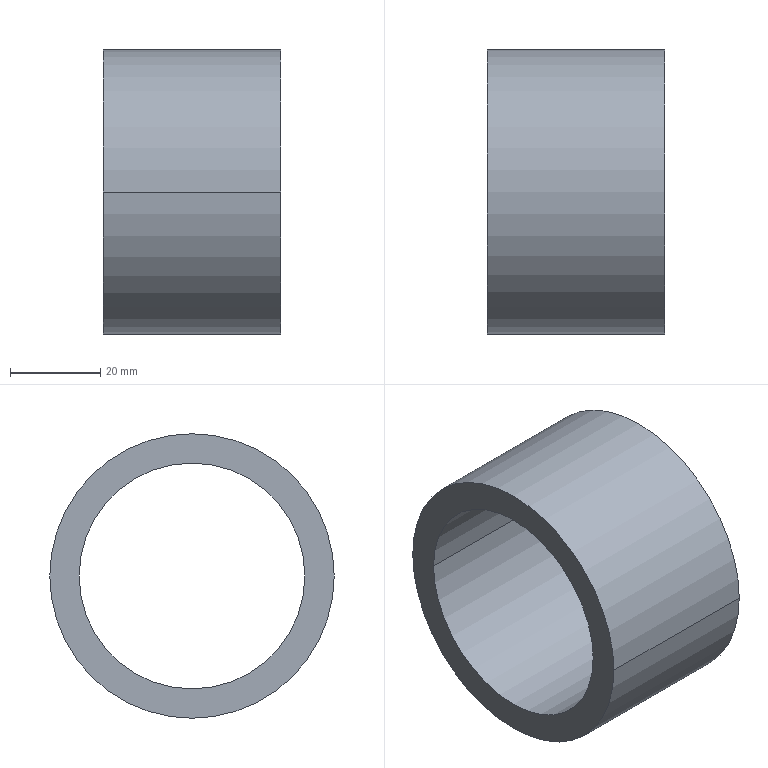Part | SolidWorks | features Extrusion 1 | 1 solid | 6 faces | box 39.25 x 63 x 63 mm | volume 45285 mm3 | cylinder 4 | plane 2 | commonest cylinder face diameters 50 x2 63 x2
STEP:
#1=CARTESIAN_POINT('',(231.,65.,-102.5));
#2=VERTEX_POINT('',#1);
#3=CARTESIAN_POINT('',(231.,115.,-102.5));
#4=VERTEX_POINT('',#3);
#5=CARTESIAN_POINT('',(231.,90.,-102.5));
#6=DIRECTION('',(1.,0.,0.));
#7=DIRECTION('',(0.,1.,0.));
#8=AXIS2_PLACEMENT_3D('',#5,#6,#7);
#9=CIRCLE('',#8,25.);
#10=EDGE_CURVE('',#2,#4,#9,.T.);
#11=ORIENTED_EDGE('',*,*,#10,.T.);
#12=CARTESIAN_POINT('',(191.75,115.,-102.5));
#13=VERTEX_POINT('',#12);
#14=CARTESIAN_POINT('',(231.,115.,-102.5));
#15=DIRECTION('',(-1.,0.,0.));
#16=VECTOR('',#15,1000.);
#17=LINE('',#14,#16);
#18=EDGE_CURVE('',#4,#13,#17,.T.);
#19=ORIENTED_EDGE('',*,*,#18,.T.);
#20=CARTESIAN_POINT('',(191.75,65.,-102.5));
#21=VERTEX_POINT('',#20);
#22=CARTESIAN_POINT('',(191.75,90.,-102.5));
#23=DIRECTION('',(1.,0.,0.));
#24=DIRECTION('',(0.,1.,0.));
#25=AXIS2_PLACEMENT_3D('',#22,#23,#24);
#26=CIRCLE('',#25,25.);
#27=EDGE_CURVE('',#21,#13,#26,.T.);
#28=ORIENTED_EDGE('',*,*,#27,.F.);
#29=CARTESIAN_POINT('',(231.,65.,-102.5));
#30=DIRECTION('',(-1.,0.,0.));
#31=VECTOR('',#30,1000.);
#32=LINE('',#29,#31);
#33=EDGE_CURVE('',#2,#21,#32,.T.);
#34=ORIENTED_EDGE('',*,*,#33,.F.);
#35=EDGE_LOOP('',(#11,#19,#28,#34));
#36=FACE_OUTER_BOUND('',#35,.T.);
#37=CARTESIAN_POINT('',(231.,90.,-102.5));
#38=DIRECTION('',(-1.,0.,0.));
#39=DIRECTION('',(0.,-1.,0.));
#40=AXIS2_PLACEMENT_3D('',#37,#38,#39);
#41=CYLINDRICAL_SURFACE('',#40,25.);
#42=ADVANCED_FACE('',(#36),#41,.F.);
#43=CARTESIAN_POINT('',(231.,121.5,-102.5));
#44=VERTEX_POINT('',#43);
#45=CARTESIAN_POINT('',(231.,58.5,-102.5));
#46=VERTEX_POINT('',#45);
#47=CARTESIAN_POINT('',(231.,90.,-102.5));
#48=DIRECTION('',(1.,0.,0.));
#49=DIRECTION('',(0.,1.,0.));
#50=AXIS2_PLACEMENT_3D('',#47,#48,#49);
#51=CIRCLE('',#50,31.5);
#52=EDGE_CURVE('',#44,#46,#51,.T.);
#53=ORIENTED_EDGE('',*,*,#52,.F.);
#54=CARTESIAN_POINT('',(191.75,121.5,-102.5));
#55=VERTEX_POINT('',#54);
#56=CARTESIAN_POINT('',(231.,121.5,-102.5));
#57=DIRECTION('',(-1.,0.,0.));
#58=VECTOR('',#57,1000.);
#59=LINE('',#56,#58);
#60=EDGE_CURVE('',#44,#55,#59,.T.);
#61=ORIENTED_EDGE('',*,*,#60,.T.);
#62=CARTESIAN_POINT('',(191.75,58.5,-102.5));
#63=VERTEX_POINT('',#62);
#64=CARTESIAN_POINT('',(191.75,90.,-102.5));
#65=DIRECTION('',(1.,0.,0.));
#66=DIRECTION('',(0.,1.,0.));
#67=AXIS2_PLACEMENT_3D('',#64,#65,#66);
#68=CIRCLE('',#67,31.5);
#69=EDGE_CURVE('',#55,#63,#68,.T.);
#70=ORIENTED_EDGE('',*,*,#69,.T.);
#71=CARTESIAN_POINT('',(231.,58.5,-102.5));
#72=DIRECTION('',(-1.,0.,0.));
#73=VECTOR('',#72,1000.);
#74=LINE('',#71,#73);
#75=EDGE_CURVE('',#46,#63,#74,.T.);
#76=ORIENTED_EDGE('',*,*,#75,.F.);
#77=EDGE_LOOP('',(#53,#61,#70,#76));
#78=FACE_OUTER_BOUND('',#77,.T.);
#79=CARTESIAN_POINT('',(231.,90.,-102.5));
#80=DIRECTION('',(-1.,0.,0.));
#81=DIRECTION('',(0.,-1.,0.));
#82=AXIS2_PLACEMENT_3D('',#79,#80,#81);
#83=CYLINDRICAL_SURFACE('',#82,31.5);
#84=ADVANCED_FACE('',(#78),#83,.T.);
#85=CARTESIAN_POINT('',(231.,90.,-102.5));
#86=DIRECTION('',(1.,0.,0.));
#87=DIRECTION('',(0.,1.,0.));
#88=AXIS2_PLACEMENT_3D('',#85,#86,#87);
#89=CIRCLE('',#88,31.5);
#90=EDGE_CURVE('',#46,#44,#89,.T.);
#91=ORIENTED_EDGE('',*,*,#90,.T.);
#92=ORIENTED_EDGE('',*,*,#52,.T.);
#93=EDGE_LOOP('',(#91,#92));
#94=FACE_OUTER_BOUND('',#93,.T.);
#95=ORIENTED_EDGE('',*,*,#10,.F.);
#96=CARTESIAN_POINT('',(231.,90.,-102.5));
#97=DIRECTION('',(1.,0.,0.));
#98=DIRECTION('',(0.,1.,0.));
#99=AXIS2_PLACEMENT_3D('',#96,#97,#98);
#100=CIRCLE('',#99,25.);
#101=EDGE_CURVE('',#4,#2,#100,.T.);
#102=ORIENTED_EDGE('',*,*,#101,.F.);
#103=EDGE_LOOP('',(#95,#102));
#104=FACE_BOUND('',#103,.T.);
#105=CARTESIAN_POINT('',(231.,90.,-102.5));
#106=DIRECTION('',(1.,0.,0.));
#107=DIRECTION('',(0.,1.,0.));
#108=AXIS2_PLACEMENT_3D('',#105,#106,#107);
#109=PLANE('',#108);
#110=ADVANCED_FACE('',(#94,#104),#109,.T.);
#111=CARTESIAN_POINT('',(191.75,90.,-102.5));
#112=DIRECTION('',(1.,0.,0.));
#113=DIRECTION('',(0.,1.,0.));
#114=AXIS2_PLACEMENT_3D('',#111,#112,#113);
#115=CIRCLE('',#114,31.5);
#116=EDGE_CURVE('',#63,#55,#115,.T.);
#117=ORIENTED_EDGE('',*,*,#116,.F.);
#118=ORIENTED_EDGE('',*,*,#69,.F.);
#119=EDGE_LOOP('',(#117,#118));
#120=FACE_OUTER_BOUND('',#119,.T.);
#121=ORIENTED_EDGE('',*,*,#27,.T.);
#122=CARTESIAN_POINT('',(191.75,90.,-102.5));
#123=DIRECTION('',(1.,0.,0.));
#124=DIRECTION('',(0.,1.,0.));
#125=AXIS2_PLACEMENT_3D('',#122,#123,#124);
#126=CIRCLE('',#125,25.);
#127=EDGE_CURVE('',#13,#21,#126,.T.);
#128=ORIENTED_EDGE('',*,*,#127,.T.);
#129=EDGE_LOOP('',(#121,#128));
#130=FACE_BOUND('',#129,.T.);
#131=CARTESIAN_POINT('',(191.75,90.,-102.5));
#132=DIRECTION('',(1.,0.,0.));
#133=DIRECTION('',(0.,1.,0.));
#134=AXIS2_PLACEMENT_3D('',#131,#132,#133);
#135=PLANE('',#134);
#136=ADVANCED_FACE('',(#120,#130),#135,.F.);
#137=ORIENTED_EDGE('',*,*,#60,.F.);
#138=ORIENTED_EDGE('',*,*,#90,.F.);
#139=ORIENTED_EDGE('',*,*,#75,.T.);
#140=ORIENTED_EDGE('',*,*,#116,.T.);
#141=EDGE_LOOP('',(#137,#138,#139,#140));
#142=FACE_OUTER_BOUND('',#141,.T.);
#143=CARTESIAN_POINT('',(231.,90.,-102.5));
#144=DIRECTION('',(-1.,0.,0.));
#145=DIRECTION('',(0.,-1.,0.));
#146=AXIS2_PLACEMENT_3D('',#143,#144,#145);
#147=CYLINDRICAL_SURFACE('',#146,31.5);
#148=ADVANCED_FACE('',(#142),#147,.T.);
#149=ORIENTED_EDGE('',*,*,#18,.F.);
#150=ORIENTED_EDGE('',*,*,#101,.T.);
#151=ORIENTED_EDGE('',*,*,#33,.T.);
#152=ORIENTED_EDGE('',*,*,#127,.F.);
#153=EDGE_LOOP('',(#149,#150,#151,#152));
#154=FACE_OUTER_BOUND('',#153,.T.);
#155=CARTESIAN_POINT('',(231.,90.,-102.5));
#156=DIRECTION('',(-1.,0.,0.));
#157=DIRECTION('',(0.,-1.,0.));
#158=AXIS2_PLACEMENT_3D('',#155,#156,#157);
#159=CYLINDRICAL_SURFACE('',#158,25.);
#160=ADVANCED_FACE('',(#154),#159,.F.);
#161=CLOSED_SHELL('',(#42,#84,#110,#136,#148,#160));
#162=MANIFOLD_SOLID_BREP('',#161);
#163=CARTESIAN_POINT('',(0.,0.,0.));
#164=DIRECTION('',(0.,0.,1.));
#165=DIRECTION('',(1.,0.,0.));
#166=AXIS2_PLACEMENT_3D('',#163,#164,#165);
#167=(LENGTH_UNIT()NAMED_UNIT(*)SI_UNIT(.MILLI.,.METRE.));
#168=UNCERTAINTY_MEASURE_WITH_UNIT(LENGTH_MEASURE(0.00001),#167,'','');
#169=(NAMED_UNIT(*)PLANE_ANGLE_UNIT()SI_UNIT($,.RADIAN.));
#170=(NAMED_UNIT(*)SI_UNIT($,.STERADIAN.)SOLID_ANGLE_UNIT());
#171=(GEOMETRIC_REPRESENTATION_CONTEXT(3)GLOBAL_UNCERTAINTY_ASSIGNED_CONTEXT((#168))GLOBAL_UNIT_ASSIGNED_CONTEXT((#167,#169,#170))REPRESENTATION_CONTEXT('',''));
#172=ADVANCED_BREP_SHAPE_REPRESENTATION('',(#162,#166),#171);